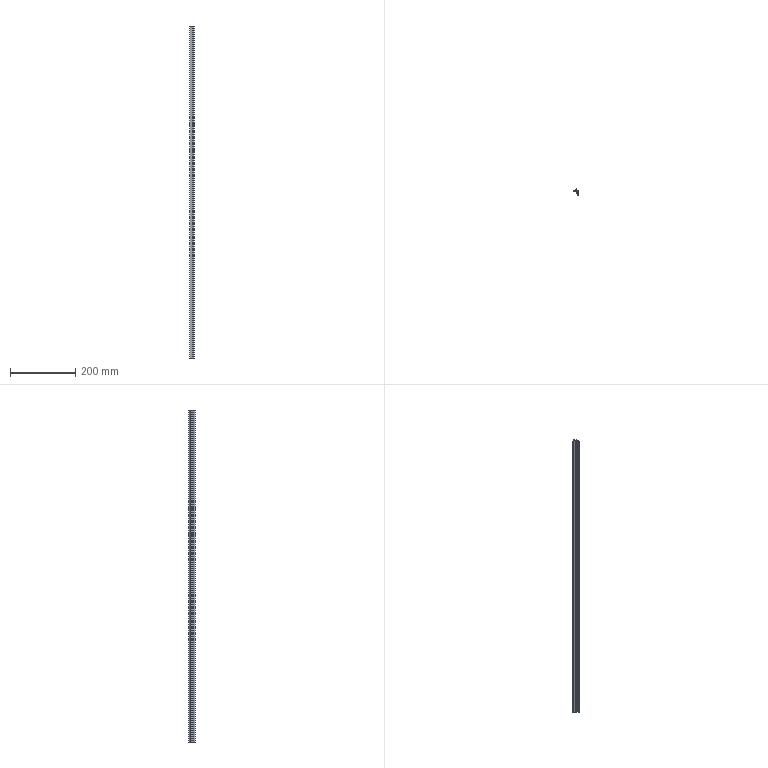Part | SolidWorks | features BaseBody 1, ICE 1, MoveFace 1 | 1 solid | 27 faces | box 14 x 20.3 x 1020 mm | volume 51934 mm3 | plane 20 | cylinder 7 | commonest cylinder face diameters 0.387 x2 0.8 x2 0.4 x1 20 x1 22 x1
STEP:
#1=CARTESIAN_POINT('',(-5.304,-0.625,200.));
#2=VERTEX_POINT('',#1);
#3=CARTESIAN_POINT('',(-5.449,-0.8125,200.));
#4=VERTEX_POINT('',#3);
#5=CARTESIAN_POINT('',(-5.255,-0.8125,200.));
#6=DIRECTION('',(0.,0.,1.));
#7=DIRECTION('',(-1.,0.,0.));
#8=AXIS2_PLACEMENT_3D('',#5,#6,#7);
#9=CIRCLE('',#8,0.1937);
#10=EDGE_CURVE('',#2,#4,#9,.T.);
#11=ORIENTED_EDGE('',*,*,#10,.T.);
#12=CARTESIAN_POINT('',(-5.449,-0.8125,-820.));
#13=VERTEX_POINT('',#12);
#14=CARTESIAN_POINT('',(-5.449,-0.8125,230.));
#15=DIRECTION('',(0.,0.,-1.));
#16=VECTOR('',#15,1000.);
#17=LINE('',#14,#16);
#18=EDGE_CURVE('',#4,#13,#17,.T.);
#19=ORIENTED_EDGE('',*,*,#18,.T.);
#20=CARTESIAN_POINT('',(-5.304,-0.625,-820.));
#21=VERTEX_POINT('',#20);
#22=CARTESIAN_POINT('',(-5.255,-0.8125,-820.));
#23=DIRECTION('',(0.,0.,-1.));
#24=DIRECTION('',(1.,0.,0.));
#25=AXIS2_PLACEMENT_3D('',#22,#23,#24);
#26=CIRCLE('',#25,0.1937);
#27=EDGE_CURVE('',#13,#21,#26,.T.);
#28=ORIENTED_EDGE('',*,*,#27,.T.);
#29=CARTESIAN_POINT('',(-5.304,-0.625,230.));
#30=DIRECTION('',(0.,0.,-1.));
#31=VECTOR('',#30,1000.);
#32=LINE('',#29,#31);
#33=EDGE_CURVE('',#2,#21,#32,.T.);
#34=ORIENTED_EDGE('',*,*,#33,.F.);
#35=EDGE_LOOP('',(#11,#19,#28,#34));
#36=FACE_OUTER_BOUND('',#35,.T.);
#37=CARTESIAN_POINT('',(-5.255,-0.8125,230.));
#38=DIRECTION('',(0.,0.,-1.));
#39=DIRECTION('',(-1.,0.,0.));
#40=AXIS2_PLACEMENT_3D('',#37,#38,#39);
#41=CYLINDRICAL_SURFACE('',#40,0.1937);
#42=ADVANCED_FACE('',(#36),#41,.F.);
#43=CARTESIAN_POINT('',(5.,-1.,-820.));
#44=VERTEX_POINT('',#43);
#45=CARTESIAN_POINT('',(5.,-14.3,-820.));
#46=VERTEX_POINT('',#45);
#47=CARTESIAN_POINT('',(5.,29.623,-820.));
#48=DIRECTION('',(0.,-1.,0.));
#49=VECTOR('',#48,1000.);
#50=LINE('',#47,#49);
#51=EDGE_CURVE('',#44,#46,#50,.T.);
#52=ORIENTED_EDGE('',*,*,#51,.F.);
#53=CARTESIAN_POINT('',(5.,-1.,200.));
#54=VERTEX_POINT('',#53);
#55=CARTESIAN_POINT('',(5.,-1.,230.));
#56=DIRECTION('',(0.,0.,-1.));
#57=VECTOR('',#56,1000.);
#58=LINE('',#55,#57);
#59=EDGE_CURVE('',#54,#44,#58,.T.);
#60=ORIENTED_EDGE('',*,*,#59,.F.);
#61=CARTESIAN_POINT('',(5.,-14.3,200.));
#62=VERTEX_POINT('',#61);
#63=CARTESIAN_POINT('',(5.,-14.3,200.));
#64=DIRECTION('',(0.,1.,0.));
#65=VECTOR('',#64,1000.);
#66=LINE('',#63,#65);
#67=EDGE_CURVE('',#62,#54,#66,.T.);
#68=ORIENTED_EDGE('',*,*,#67,.F.);
#69=CARTESIAN_POINT('',(5.,-14.3,230.));
#70=DIRECTION('',(0.,0.,1.));
#71=VECTOR('',#70,1000.);
#72=LINE('',#69,#71);
#73=EDGE_CURVE('',#46,#62,#72,.T.);
#74=ORIENTED_EDGE('',*,*,#73,.F.);
#75=EDGE_LOOP('',(#52,#60,#68,#74));
#76=FACE_OUTER_BOUND('',#75,.T.);
#77=CARTESIAN_POINT('',(5.,-14.3,230.));
#78=DIRECTION('',(-1.,0.,0.));
#79=DIRECTION('',(0.,0.,1.));
#80=AXIS2_PLACEMENT_3D('',#77,#78,#79);
#81=PLANE('',#80);
#82=ADVANCED_FACE('',(#76),#81,.F.);
#83=CARTESIAN_POINT('',(-9.,-2.,-820.));
#84=VERTEX_POINT('',#83);
#85=CARTESIAN_POINT('',(-9.,-2.,200.));
#86=VERTEX_POINT('',#85);
#87=CARTESIAN_POINT('',(-9.,-2.,230.));
#88=DIRECTION('',(0.,0.,1.));
#89=VECTOR('',#88,1000.);
#90=LINE('',#87,#89);
#91=EDGE_CURVE('',#84,#86,#90,.T.);
#92=ORIENTED_EDGE('',*,*,#91,.F.);
#93=CARTESIAN_POINT('',(0.9,-2.,-820.));
#94=VERTEX_POINT('',#93);
#95=CARTESIAN_POINT('',(5.,-2.,-820.));
#96=DIRECTION('',(-1.,0.,0.));
#97=VECTOR('',#96,1000.);
#98=LINE('',#95,#97);
#99=EDGE_CURVE('',#94,#84,#98,.T.);
#100=ORIENTED_EDGE('',*,*,#99,.F.);
#101=CARTESIAN_POINT('',(0.9,-2.,200.));
#102=VERTEX_POINT('',#101);
#103=CARTESIAN_POINT('',(0.9,-2.,230.));
#104=DIRECTION('',(0.,0.,-1.));
#105=VECTOR('',#104,1000.);
#106=LINE('',#103,#105);
#107=EDGE_CURVE('',#102,#94,#106,.T.);
#108=ORIENTED_EDGE('',*,*,#107,.F.);
#109=CARTESIAN_POINT('',(5.,-2.,200.));
#110=DIRECTION('',(1.,0.,0.));
#111=VECTOR('',#110,1000.);
#112=LINE('',#109,#111);
#113=EDGE_CURVE('',#86,#102,#112,.T.);
#114=ORIENTED_EDGE('',*,*,#113,.F.);
#115=EDGE_LOOP('',(#92,#100,#108,#114));
#116=FACE_OUTER_BOUND('',#115,.T.);
#117=CARTESIAN_POINT('',(-9.,-2.,230.));
#118=DIRECTION('',(0.,1.,0.));
#119=DIRECTION('',(0.,0.,1.));
#120=AXIS2_PLACEMENT_3D('',#117,#118,#119);
#121=PLANE('',#120);
#122=ADVANCED_FACE('',(#116),#121,.F.);
#123=CARTESIAN_POINT('',(4.,-6.,200.));
#124=VERTEX_POINT('',#123);
#125=CARTESIAN_POINT('',(4.,-3.,200.));
#126=VERTEX_POINT('',#125);
#127=CARTESIAN_POINT('',(4.,29.623,200.));
#128=DIRECTION('',(0.,1.,0.));
#129=VECTOR('',#128,1000.);
#130=LINE('',#127,#129);
#131=EDGE_CURVE('',#124,#126,#130,.T.);
#132=ORIENTED_EDGE('',*,*,#131,.F.);
#133=CARTESIAN_POINT('',(1.,-6.,200.));
#134=VERTEX_POINT('',#133);
#135=CARTESIAN_POINT('',(5.,-6.,200.));
#136=DIRECTION('',(1.,0.,0.));
#137=VECTOR('',#136,1000.);
#138=LINE('',#135,#137);
#139=EDGE_CURVE('',#134,#124,#138,.T.);
#140=ORIENTED_EDGE('',*,*,#139,.F.);
#141=CARTESIAN_POINT('',(1.,-6.7,200.));
#142=VERTEX_POINT('',#141);
#143=CARTESIAN_POINT('',(1.,-6.,200.));
#144=DIRECTION('',(0.,-1.,0.));
#145=VECTOR('',#144,1000.);
#146=LINE('',#143,#145);
#147=EDGE_CURVE('',#134,#142,#146,.T.);
#148=ORIENTED_EDGE('',*,*,#147,.T.);
#149=CARTESIAN_POINT('',(-1.7,-6.7,200.));
#150=VERTEX_POINT('',#149);
#151=CARTESIAN_POINT('',(5.,-6.7,200.));
#152=DIRECTION('',(1.,0.,0.));
#153=VECTOR('',#152,1000.);
#154=LINE('',#151,#153);
#155=EDGE_CURVE('',#150,#142,#154,.T.);
#156=ORIENTED_EDGE('',*,*,#155,.F.);
#157=CARTESIAN_POINT('',(-1.7,-7.7,200.));
#158=VERTEX_POINT('',#157);
#159=CARTESIAN_POINT('',(-1.7,-6.7,200.));
#160=DIRECTION('',(0.,-1.,0.));
#161=VECTOR('',#160,1000.);
#162=LINE('',#159,#161);
#163=EDGE_CURVE('',#150,#158,#162,.T.);
#164=ORIENTED_EDGE('',*,*,#163,.T.);
#165=CARTESIAN_POINT('',(4.,-7.7,200.));
#166=VERTEX_POINT('',#165);
#167=CARTESIAN_POINT('',(5.,-7.7,200.));
#168=DIRECTION('',(-1.,0.,0.));
#169=VECTOR('',#168,1000.);
#170=LINE('',#167,#169);
#171=EDGE_CURVE('',#166,#158,#170,.T.);
#172=ORIENTED_EDGE('',*,*,#171,.F.);
#173=CARTESIAN_POINT('',(4.,-14.3,200.));
#174=VERTEX_POINT('',#173);
#175=CARTESIAN_POINT('',(4.,29.623,200.));
#176=DIRECTION('',(0.,1.,0.));
#177=VECTOR('',#176,1000.);
#178=LINE('',#175,#177);
#179=EDGE_CURVE('',#174,#166,#178,.T.);
#180=ORIENTED_EDGE('',*,*,#179,.F.);
#181=CARTESIAN_POINT('',(5.,-14.3,200.));
#182=DIRECTION('',(-1.,0.,0.));
#183=VECTOR('',#182,1000.);
#184=LINE('',#181,#183);
#185=EDGE_CURVE('',#62,#174,#184,.T.);
#186=ORIENTED_EDGE('',*,*,#185,.F.);
#187=ORIENTED_EDGE('',*,*,#67,.T.);
#188=CARTESIAN_POINT('',(-5.207,-1.,200.));
#189=VERTEX_POINT('',#188);
#190=CARTESIAN_POINT('',(5.,-1.,200.));
#191=DIRECTION('',(1.,0.,0.));
#192=VECTOR('',#191,1000.);
#193=LINE('',#190,#192);
#194=EDGE_CURVE('',#189,#54,#193,.T.);
#195=ORIENTED_EDGE('',*,*,#194,.F.);
#196=CARTESIAN_POINT('',(-5.255,-0.8125,200.));
#197=DIRECTION('',(0.,0.,1.));
#198=DIRECTION('',(-1.,0.,0.));
#199=AXIS2_PLACEMENT_3D('',#196,#197,#198);
#200=CIRCLE('',#199,0.1937);
#201=EDGE_CURVE('',#4,#189,#200,.T.);
#202=ORIENTED_EDGE('',*,*,#201,.F.);
#203=ORIENTED_EDGE('',*,*,#10,.F.);
#204=CARTESIAN_POINT('',(-1.368,3.063,200.));
#205=VERTEX_POINT('',#204);
#206=CARTESIAN_POINT('',(-10.628,9.,200.));
#207=DIRECTION('',(0.,0.,1.));
#208=DIRECTION('',(-1.,0.,0.));
#209=AXIS2_PLACEMENT_3D('',#206,#207,#208);
#210=CIRCLE('',#209,11.);
#211=EDGE_CURVE('',#2,#205,#210,.T.);
#212=ORIENTED_EDGE('',*,*,#211,.T.);
#213=CARTESIAN_POINT('',(-1.,2.955,200.));
#214=VERTEX_POINT('',#213);
#215=CARTESIAN_POINT('',(-1.2,2.955,200.));
#216=DIRECTION('',(0.,0.,1.));
#217=DIRECTION('',(-1.,0.,0.));
#218=AXIS2_PLACEMENT_3D('',#215,#216,#217);
#219=CIRCLE('',#218,0.2);
#220=EDGE_CURVE('',#214,#205,#219,.T.);
#221=ORIENTED_EDGE('',*,*,#220,.F.);
#222=CARTESIAN_POINT('',(-1.,1.5,200.));
#223=VERTEX_POINT('',#222);
#224=CARTESIAN_POINT('',(-1.,2.955,200.));
#225=DIRECTION('',(0.,1.,0.));
#226=VECTOR('',#225,1000.);
#227=LINE('',#224,#226);
#228=EDGE_CURVE('',#223,#214,#227,.T.);
#229=ORIENTED_EDGE('',*,*,#228,.F.);
#230=CARTESIAN_POINT('',(0.,1.5,200.));
#231=VERTEX_POINT('',#230);
#232=CARTESIAN_POINT('',(-1.,1.5,200.));
#233=DIRECTION('',(-1.,0.,0.));
#234=VECTOR('',#233,1000.);
#235=LINE('',#232,#234);
#236=EDGE_CURVE('',#231,#223,#235,.T.);
#237=ORIENTED_EDGE('',*,*,#236,.F.);
#238=CARTESIAN_POINT('',(0.,6.,200.));
#239=VERTEX_POINT('',#238);
#240=CARTESIAN_POINT('',(0.,1.5,200.));
#241=DIRECTION('',(0.,-1.,0.));
#242=VECTOR('',#241,1000.);
#243=LINE('',#240,#242);
#244=EDGE_CURVE('',#239,#231,#243,.T.);
#245=ORIENTED_EDGE('',*,*,#244,.F.);
#246=CARTESIAN_POINT('',(-0.8,6.,200.));
#247=VERTEX_POINT('',#246);
#248=CARTESIAN_POINT('',(0.,6.,200.));
#249=DIRECTION('',(1.,0.,0.));
#250=VECTOR('',#249,1000.);
#251=LINE('',#248,#250);
#252=EDGE_CURVE('',#247,#239,#251,.T.);
#253=ORIENTED_EDGE('',*,*,#252,.F.);
#254=CARTESIAN_POINT('',(-1.178,5.731,200.));
#255=VERTEX_POINT('',#254);
#256=CARTESIAN_POINT('',(-0.8,5.6,200.));
#257=DIRECTION('',(0.,0.,1.));
#258=DIRECTION('',(-1.,0.,0.));
#259=AXIS2_PLACEMENT_3D('',#256,#257,#258);
#260=CIRCLE('',#259,0.4);
#261=EDGE_CURVE('',#247,#255,#260,.T.);
#262=ORIENTED_EDGE('',*,*,#261,.T.);
#263=CARTESIAN_POINT('',(-8.678,-0.8077,200.));
#264=VERTEX_POINT('',#263);
#265=CARTESIAN_POINT('',(-10.628,9.,200.));
#266=DIRECTION('',(0.,0.,1.));
#267=DIRECTION('',(-1.,0.,0.));
#268=AXIS2_PLACEMENT_3D('',#265,#266,#267);
#269=CIRCLE('',#268,10.);
#270=EDGE_CURVE('',#264,#255,#269,.T.);
#271=ORIENTED_EDGE('',*,*,#270,.F.);
#272=CARTESIAN_POINT('',(-9.,-1.2,200.));
#273=VERTEX_POINT('',#272);
#274=CARTESIAN_POINT('',(-8.6,-1.2,200.));
#275=DIRECTION('',(0.,0.,1.));
#276=DIRECTION('',(-1.,0.,0.));
#277=AXIS2_PLACEMENT_3D('',#274,#275,#276);
#278=CIRCLE('',#277,0.4);
#279=EDGE_CURVE('',#264,#273,#278,.T.);
#280=ORIENTED_EDGE('',*,*,#279,.T.);
#281=CARTESIAN_POINT('',(-9.,8.,200.));
#282=DIRECTION('',(0.,-1.,0.));
#283=VECTOR('',#282,1000.);
#284=LINE('',#281,#283);
#285=EDGE_CURVE('',#273,#86,#284,.T.);
#286=ORIENTED_EDGE('',*,*,#285,.T.);
#287=ORIENTED_EDGE('',*,*,#113,.T.);
#288=CARTESIAN_POINT('',(0.9,-3.,200.));
#289=VERTEX_POINT('',#288);
#290=CARTESIAN_POINT('',(0.9,29.623,200.));
#291=DIRECTION('',(0.,1.,0.));
#292=VECTOR('',#291,1000.);
#293=LINE('',#290,#292);
#294=EDGE_CURVE('',#289,#102,#293,.T.);
#295=ORIENTED_EDGE('',*,*,#294,.F.);
#296=CARTESIAN_POINT('',(5.,-3.,200.));
#297=DIRECTION('',(-1.,0.,0.));
#298=VECTOR('',#297,1000.);
#299=LINE('',#296,#298);
#300=EDGE_CURVE('',#126,#289,#299,.T.);
#301=ORIENTED_EDGE('',*,*,#300,.F.);
#302=EDGE_LOOP('',(#132,#140,#148,#156,#164,#172,#180,#186,#187,#195,#202,#203,#212,#221,#229,#237,#245,#253,#262,#271,#280,#286,#287,#295,#301));
#303=FACE_OUTER_BOUND('',#302,.T.);
#304=CARTESIAN_POINT('',(5.,29.623,200.));
#305=DIRECTION('',(0.,0.,-1.));
#306=DIRECTION('',(-1.,0.,0.));
#307=AXIS2_PLACEMENT_3D('',#304,#305,#306);
#308=PLANE('',#307);
#309=ADVANCED_FACE('',(#303),#308,.F.);
#310=ORIENTED_EDGE('',*,*,#185,.T.);
#311=CARTESIAN_POINT('',(4.,-14.3,-820.));
#312=VERTEX_POINT('',#311);
#313=CARTESIAN_POINT('',(4.,-14.3,230.));
#314=DIRECTION('',(0.,0.,1.));
#315=VECTOR('',#314,1000.);
#316=LINE('',#313,#315);
#317=EDGE_CURVE('',#312,#174,#316,.T.);
#318=ORIENTED_EDGE('',*,*,#317,.F.);
#319=CARTESIAN_POINT('',(5.,-14.3,-820.));
#320=DIRECTION('',(-1.,0.,0.));
#321=VECTOR('',#320,1000.);
#322=LINE('',#319,#321);
#323=EDGE_CURVE('',#46,#312,#322,.T.);
#324=ORIENTED_EDGE('',*,*,#323,.F.);
#325=ORIENTED_EDGE('',*,*,#73,.T.);
#326=EDGE_LOOP('',(#310,#318,#324,#325));
#327=FACE_OUTER_BOUND('',#326,.T.);
#328=CARTESIAN_POINT('',(4.,-14.3,230.));
#329=DIRECTION('',(0.,1.,0.));
#330=DIRECTION('',(0.,0.,1.));
#331=AXIS2_PLACEMENT_3D('',#328,#329,#330);
#332=PLANE('',#331);
#333=ADVANCED_FACE('',(#327),#332,.F.);
#334=ORIENTED_EDGE('',*,*,#51,.T.);
#335=ORIENTED_EDGE('',*,*,#323,.T.);
#336=CARTESIAN_POINT('',(4.,-7.7,-820.));
#337=VERTEX_POINT('',#336);
#338=CARTESIAN_POINT('',(4.,-7.7,-820.));
#339=DIRECTION('',(0.,-1.,0.));
#340=VECTOR('',#339,1000.);
#341=LINE('',#338,#340);
#342=EDGE_CURVE('',#337,#312,#341,.T.);
#343=ORIENTED_EDGE('',*,*,#342,.F.);
#344=CARTESIAN_POINT('',(-1.7,-7.7,-820.));
#345=VERTEX_POINT('',#344);
#346=CARTESIAN_POINT('',(-1.7,-7.7,-820.));
#347=DIRECTION('',(1.,0.,0.));
#348=VECTOR('',#347,1000.);
#349=LINE('',#346,#348);
#350=EDGE_CURVE('',#345,#337,#349,.T.);
#351=ORIENTED_EDGE('',*,*,#350,.F.);
#352=CARTESIAN_POINT('',(-1.7,-6.7,-820.));
#353=VERTEX_POINT('',#352);
#354=CARTESIAN_POINT('',(-1.7,29.623,-820.));
#355=DIRECTION('',(0.,1.,0.));
#356=VECTOR('',#355,1000.);
#357=LINE('',#354,#356);
#358=EDGE_CURVE('',#345,#353,#357,.T.);
#359=ORIENTED_EDGE('',*,*,#358,.T.);
#360=CARTESIAN_POINT('',(1.,-6.7,-820.));
#361=VERTEX_POINT('',#360);
#362=CARTESIAN_POINT('',(1.,-6.7,-820.));
#363=DIRECTION('',(-1.,0.,0.));
#364=VECTOR('',#363,1000.);
#365=LINE('',#362,#364);
#366=EDGE_CURVE('',#361,#353,#365,.T.);
#367=ORIENTED_EDGE('',*,*,#366,.F.);
#368=CARTESIAN_POINT('',(1.,-6.,-820.));
#369=VERTEX_POINT('',#368);
#370=CARTESIAN_POINT('',(1.,29.623,-820.));
#371=DIRECTION('',(0.,1.,0.));
#372=VECTOR('',#371,1000.);
#373=LINE('',#370,#372);
#374=EDGE_CURVE('',#361,#369,#373,.T.);
#375=ORIENTED_EDGE('',*,*,#374,.T.);
#376=CARTESIAN_POINT('',(4.,-6.,-820.));
#377=VERTEX_POINT('',#376);
#378=CARTESIAN_POINT('',(4.,-6.,-820.));
#379=DIRECTION('',(-1.,0.,0.));
#380=VECTOR('',#379,1000.);
#381=LINE('',#378,#380);
#382=EDGE_CURVE('',#377,#369,#381,.T.);
#383=ORIENTED_EDGE('',*,*,#382,.F.);
#384=CARTESIAN_POINT('',(4.,-3.,-820.));
#385=VERTEX_POINT('',#384);
#386=CARTESIAN_POINT('',(4.,-3.,-820.));
#387=DIRECTION('',(0.,-1.,0.));
#388=VECTOR('',#387,1000.);
#389=LINE('',#386,#388);
#390=EDGE_CURVE('',#385,#377,#389,.T.);
#391=ORIENTED_EDGE('',*,*,#390,.F.);
#392=CARTESIAN_POINT('',(0.9,-3.,-820.));
#393=VERTEX_POINT('',#392);
#394=CARTESIAN_POINT('',(0.9,-3.,-820.));
#395=DIRECTION('',(1.,0.,0.));
#396=VECTOR('',#395,1000.);
#397=LINE('',#394,#396);
#398=EDGE_CURVE('',#393,#385,#397,.T.);
#399=ORIENTED_EDGE('',*,*,#398,.F.);
#400=CARTESIAN_POINT('',(0.9,-2.,-820.));
#401=DIRECTION('',(0.,-1.,0.));
#402=VECTOR('',#401,1000.);
#403=LINE('',#400,#402);
#404=EDGE_CURVE('',#94,#393,#403,.T.);
#405=ORIENTED_EDGE('',*,*,#404,.F.);
#406=ORIENTED_EDGE('',*,*,#99,.T.);
#407=CARTESIAN_POINT('',(-9.,-1.2,-820.));
#408=VERTEX_POINT('',#407);
#409=CARTESIAN_POINT('',(-9.,-1.2,-820.));
#410=DIRECTION('',(0.,-1.,0.));
#411=VECTOR('',#410,1000.);
#412=LINE('',#409,#411);
#413=EDGE_CURVE('',#408,#84,#412,.T.);
#414=ORIENTED_EDGE('',*,*,#413,.F.);
#415=CARTESIAN_POINT('',(-8.678,-0.8077,-820.));
#416=VERTEX_POINT('',#415);
#417=CARTESIAN_POINT('',(-8.6,-1.2,-820.));
#418=DIRECTION('',(0.,0.,-1.));
#419=DIRECTION('',(1.,0.,0.));
#420=AXIS2_PLACEMENT_3D('',#417,#418,#419);
#421=CIRCLE('',#420,0.4);
#422=EDGE_CURVE('',#408,#416,#421,.T.);
#423=ORIENTED_EDGE('',*,*,#422,.T.);
#424=CARTESIAN_POINT('',(-1.178,5.731,-820.));
#425=VERTEX_POINT('',#424);
#426=CARTESIAN_POINT('',(-10.628,9.,-820.));
#427=DIRECTION('',(0.,0.,-1.));
#428=DIRECTION('',(1.,0.,0.));
#429=AXIS2_PLACEMENT_3D('',#426,#427,#428);
#430=CIRCLE('',#429,10.);
#431=EDGE_CURVE('',#425,#416,#430,.T.);
#432=ORIENTED_EDGE('',*,*,#431,.F.);
#433=CARTESIAN_POINT('',(-0.8,6.,-820.));
#434=VERTEX_POINT('',#433);
#435=CARTESIAN_POINT('',(-0.8,5.6,-820.));
#436=DIRECTION('',(0.,0.,-1.));
#437=DIRECTION('',(1.,0.,0.));
#438=AXIS2_PLACEMENT_3D('',#435,#436,#437);
#439=CIRCLE('',#438,0.4);
#440=EDGE_CURVE('',#425,#434,#439,.T.);
#441=ORIENTED_EDGE('',*,*,#440,.T.);
#442=CARTESIAN_POINT('',(0.,6.,-820.));
#443=VERTEX_POINT('',#442);
#444=CARTESIAN_POINT('',(0.,6.,-820.));
#445=DIRECTION('',(-1.,0.,0.));
#446=VECTOR('',#445,1000.);
#447=LINE('',#444,#446);
#448=EDGE_CURVE('',#443,#434,#447,.T.);
#449=ORIENTED_EDGE('',*,*,#448,.F.);
#450=CARTESIAN_POINT('',(0.,1.5,-820.));
#451=VERTEX_POINT('',#450);
#452=CARTESIAN_POINT('',(0.,1.5,-820.));
#453=DIRECTION('',(0.,1.,0.));
#454=VECTOR('',#453,1000.);
#455=LINE('',#452,#454);
#456=EDGE_CURVE('',#451,#443,#455,.T.);
#457=ORIENTED_EDGE('',*,*,#456,.F.);
#458=CARTESIAN_POINT('',(-1.,1.5,-820.));
#459=VERTEX_POINT('',#458);
#460=CARTESIAN_POINT('',(-1.,1.5,-820.));
#461=DIRECTION('',(1.,0.,0.));
#462=VECTOR('',#461,1000.);
#463=LINE('',#460,#462);
#464=EDGE_CURVE('',#459,#451,#463,.T.);
#465=ORIENTED_EDGE('',*,*,#464,.F.);
#466=CARTESIAN_POINT('',(-1.,2.955,-820.));
#467=VERTEX_POINT('',#466);
#468=CARTESIAN_POINT('',(-1.,2.955,-820.));
#469=DIRECTION('',(0.,-1.,0.));
#470=VECTOR('',#469,1000.);
#471=LINE('',#468,#470);
#472=EDGE_CURVE('',#467,#459,#471,.T.);
#473=ORIENTED_EDGE('',*,*,#472,.F.);
#474=CARTESIAN_POINT('',(-1.368,3.063,-820.));
#475=VERTEX_POINT('',#474);
#476=CARTESIAN_POINT('',(-1.2,2.955,-820.));
#477=DIRECTION('',(0.,0.,-1.));
#478=DIRECTION('',(1.,0.,0.));
#479=AXIS2_PLACEMENT_3D('',#476,#477,#478);
#480=CIRCLE('',#479,0.2);
#481=EDGE_CURVE('',#475,#467,#480,.T.);
#482=ORIENTED_EDGE('',*,*,#481,.F.);
#483=CARTESIAN_POINT('',(-10.628,9.,-820.));
#484=DIRECTION('',(0.,0.,-1.));
#485=DIRECTION('',(1.,0.,0.));
#486=AXIS2_PLACEMENT_3D('',#483,#484,#485);
#487=CIRCLE('',#486,11.);
#488=EDGE_CURVE('',#475,#21,#487,.T.);
#489=ORIENTED_EDGE('',*,*,#488,.T.);
#490=ORIENTED_EDGE('',*,*,#27,.F.);
#491=CARTESIAN_POINT('',(-5.207,-1.,-820.));
#492=VERTEX_POINT('',#491);
#493=CARTESIAN_POINT('',(-5.255,-0.8125,-820.));
#494=DIRECTION('',(0.,0.,-1.));
#495=DIRECTION('',(1.,0.,0.));
#496=AXIS2_PLACEMENT_3D('',#493,#494,#495);
#497=CIRCLE('',#496,0.1937);
#498=EDGE_CURVE('',#492,#13,#497,.T.);
#499=ORIENTED_EDGE('',*,*,#498,.F.);
#500=CARTESIAN_POINT('',(5.,-1.,-820.));
#501=DIRECTION('',(-1.,0.,0.));
#502=VECTOR('',#501,1000.);
#503=LINE('',#500,#502);
#504=EDGE_CURVE('',#44,#492,#503,.T.);
#505=ORIENTED_EDGE('',*,*,#504,.F.);
#506=EDGE_LOOP('',(#334,#335,#343,#351,#359,#367,#375,#383,#391,#399,#405,#406,#414,#423,#432,#441,#449,#457,#465,#473,#482,#489,#490,#499,#505));
#507=FACE_OUTER_BOUND('',#506,.T.);
#508=CARTESIAN_POINT('',(5.,29.623,-820.));
#509=DIRECTION('',(0.,0.,1.));
#510=DIRECTION('',(1.,0.,0.));
#511=AXIS2_PLACEMENT_3D('',#508,#509,#510);
#512=PLANE('',#511);
#513=ADVANCED_FACE('',(#507),#512,.F.);
#514=ORIENTED_EDGE('',*,*,#59,.T.);
#515=ORIENTED_EDGE('',*,*,#504,.T.);
#516=CARTESIAN_POINT('',(-5.207,-1.,230.));
#517=DIRECTION('',(0.,0.,-1.));
#518=VECTOR('',#517,1000.);
#519=LINE('',#516,#518);
#520=EDGE_CURVE('',#189,#492,#519,.T.);
#521=ORIENTED_EDGE('',*,*,#520,.F.);
#522=ORIENTED_EDGE('',*,*,#194,.T.);
#523=EDGE_LOOP('',(#514,#515,#521,#522));
#524=FACE_OUTER_BOUND('',#523,.T.);
#525=CARTESIAN_POINT('',(5.,-1.,230.));
#526=DIRECTION('',(0.,-1.,0.));
#527=DIRECTION('',(0.,0.,-1.));
#528=AXIS2_PLACEMENT_3D('',#525,#526,#527);
#529=PLANE('',#528);
#530=ADVANCED_FACE('',(#524),#529,.F.);
#531=CARTESIAN_POINT('',(-9.,-1.2,230.));
#532=DIRECTION('',(0.,0.,1.));
#533=VECTOR('',#532,1000.);
#534=LINE('',#531,#533);
#535=EDGE_CURVE('',#408,#273,#534,.T.);
#536=ORIENTED_EDGE('',*,*,#535,.F.);
#537=ORIENTED_EDGE('',*,*,#413,.T.);
#538=ORIENTED_EDGE('',*,*,#91,.T.);
#539=ORIENTED_EDGE('',*,*,#285,.F.);
#540=EDGE_LOOP('',(#536,#537,#538,#539));
#541=FACE_OUTER_BOUND('',#540,.T.);
#542=CARTESIAN_POINT('',(-9.,-1.2,230.));
#543=DIRECTION('',(1.,0.,0.));
#544=DIRECTION('',(0.,0.,-1.));
#545=AXIS2_PLACEMENT_3D('',#542,#543,#544);
#546=PLANE('',#545);
#547=ADVANCED_FACE('',(#541),#546,.F.);
#548=ORIENTED_EDGE('',*,*,#294,.T.);
#549=ORIENTED_EDGE('',*,*,#107,.T.);
#550=ORIENTED_EDGE('',*,*,#404,.T.);
#551=CARTESIAN_POINT('',(0.9,-3.,230.));
#552=DIRECTION('',(0.,0.,-1.));
#553=VECTOR('',#552,1000.);
#554=LINE('',#551,#553);
#555=EDGE_CURVE('',#289,#393,#554,.T.);
#556=ORIENTED_EDGE('',*,*,#555,.F.);
#557=EDGE_LOOP('',(#548,#549,#550,#556));
#558=FACE_OUTER_BOUND('',#557,.T.);
#559=CARTESIAN_POINT('',(0.9,-2.,230.));
#560=DIRECTION('',(1.,0.,0.));
#561=DIRECTION('',(0.,0.,-1.));
#562=AXIS2_PLACEMENT_3D('',#559,#560,#561);
#563=PLANE('',#562);
#564=ADVANCED_FACE('',(#558),#563,.F.);
#565=ORIENTED_EDGE('',*,*,#300,.T.);
#566=ORIENTED_EDGE('',*,*,#555,.T.);
#567=ORIENTED_EDGE('',*,*,#398,.T.);
#568=CARTESIAN_POINT('',(4.,-3.,230.));
#569=DIRECTION('',(0.,0.,-1.));
#570=VECTOR('',#569,1000.);
#571=LINE('',#568,#570);
#572=EDGE_CURVE('',#126,#385,#571,.T.);
#573=ORIENTED_EDGE('',*,*,#572,.F.);
#574=EDGE_LOOP('',(#565,#566,#567,#573));
#575=FACE_OUTER_BOUND('',#574,.T.);
#576=CARTESIAN_POINT('',(0.9,-3.,230.));
#577=DIRECTION('',(0.,1.,0.));
#578=DIRECTION('',(0.,0.,1.));
#579=AXIS2_PLACEMENT_3D('',#576,#577,#578);
#580=PLANE('',#579);
#581=ADVANCED_FACE('',(#575),#580,.F.);
#582=ORIENTED_EDGE('',*,*,#131,.T.);
#583=ORIENTED_EDGE('',*,*,#572,.T.);
#584=ORIENTED_EDGE('',*,*,#390,.T.);
#585=CARTESIAN_POINT('',(4.,-6.,230.));
#586=DIRECTION('',(0.,0.,-1.));
#587=VECTOR('',#586,1000.);
#588=LINE('',#585,#587);
#589=EDGE_CURVE('',#124,#377,#588,.T.);
#590=ORIENTED_EDGE('',*,*,#589,.F.);
#591=EDGE_LOOP('',(#582,#583,#584,#590));
#592=FACE_OUTER_BOUND('',#591,.T.);
#593=CARTESIAN_POINT('',(4.,-3.,230.));
#594=DIRECTION('',(1.,0.,0.));
#595=DIRECTION('',(0.,0.,-1.));
#596=AXIS2_PLACEMENT_3D('',#593,#594,#595);
#597=PLANE('',#596);
#598=ADVANCED_FACE('',(#592),#597,.F.);
#599=ORIENTED_EDGE('',*,*,#139,.T.);
#600=ORIENTED_EDGE('',*,*,#589,.T.);
#601=ORIENTED_EDGE('',*,*,#382,.T.);
#602=CARTESIAN_POINT('',(1.,-6.,230.));
#603=DIRECTION('',(0.,0.,-1.));
#604=VECTOR('',#603,1000.);
#605=LINE('',#602,#604);
#606=EDGE_CURVE('',#134,#369,#605,.T.);
#607=ORIENTED_EDGE('',*,*,#606,.F.);
#608=EDGE_LOOP('',(#599,#600,#601,#607));
#609=FACE_OUTER_BOUND('',#608,.T.);
#610=CARTESIAN_POINT('',(4.,-6.,230.));
#611=DIRECTION('',(0.,-1.,0.));
#612=DIRECTION('',(0.,0.,-1.));
#613=AXIS2_PLACEMENT_3D('',#610,#611,#612);
#614=PLANE('',#613);
#615=ADVANCED_FACE('',(#609),#614,.F.);
#616=ORIENTED_EDGE('',*,*,#155,.T.);
#617=CARTESIAN_POINT('',(1.,-6.7,230.));
#618=DIRECTION('',(0.,0.,1.));
#619=VECTOR('',#618,1000.);
#620=LINE('',#617,#619);
#621=EDGE_CURVE('',#361,#142,#620,.T.);
#622=ORIENTED_EDGE('',*,*,#621,.F.);
#623=ORIENTED_EDGE('',*,*,#366,.T.);
#624=CARTESIAN_POINT('',(-1.7,-6.7,230.));
#625=DIRECTION('',(0.,0.,-1.));
#626=VECTOR('',#625,1000.);
#627=LINE('',#624,#626);
#628=EDGE_CURVE('',#150,#353,#627,.T.);
#629=ORIENTED_EDGE('',*,*,#628,.F.);
#630=EDGE_LOOP('',(#616,#622,#623,#629));
#631=FACE_OUTER_BOUND('',#630,.T.);
#632=CARTESIAN_POINT('',(1.,-6.7,230.));
#633=DIRECTION('',(0.,-1.,0.));
#634=DIRECTION('',(0.,0.,-1.));
#635=AXIS2_PLACEMENT_3D('',#632,#633,#634);
#636=PLANE('',#635);
#637=ADVANCED_FACE('',(#631),#636,.F.);
#638=ORIENTED_EDGE('',*,*,#171,.T.);
#639=CARTESIAN_POINT('',(-1.7,-7.7,230.));
#640=DIRECTION('',(0.,0.,1.));
#641=VECTOR('',#640,1000.);
#642=LINE('',#639,#641);
#643=EDGE_CURVE('',#345,#158,#642,.T.);
#644=ORIENTED_EDGE('',*,*,#643,.F.);
#645=ORIENTED_EDGE('',*,*,#350,.T.);
#646=CARTESIAN_POINT('',(4.,-7.7,230.));
#647=DIRECTION('',(0.,0.,-1.));
#648=VECTOR('',#647,1000.);
#649=LINE('',#646,#648);
#650=EDGE_CURVE('',#166,#337,#649,.T.);
#651=ORIENTED_EDGE('',*,*,#650,.F.);
#652=EDGE_LOOP('',(#638,#644,#645,#651));
#653=FACE_OUTER_BOUND('',#652,.T.);
#654=CARTESIAN_POINT('',(-1.7,-7.7,230.));
#655=DIRECTION('',(0.,1.,0.));
#656=DIRECTION('',(0.,0.,1.));
#657=AXIS2_PLACEMENT_3D('',#654,#655,#656);
#658=PLANE('',#657);
#659=ADVANCED_FACE('',(#653),#658,.F.);
#660=ORIENTED_EDGE('',*,*,#179,.T.);
#661=ORIENTED_EDGE('',*,*,#650,.T.);
#662=ORIENTED_EDGE('',*,*,#342,.T.);
#663=ORIENTED_EDGE('',*,*,#317,.T.);
#664=EDGE_LOOP('',(#660,#661,#662,#663));
#665=FACE_OUTER_BOUND('',#664,.T.);
#666=CARTESIAN_POINT('',(4.,-7.7,230.));
#667=DIRECTION('',(1.,0.,0.));
#668=DIRECTION('',(0.,0.,-1.));
#669=AXIS2_PLACEMENT_3D('',#666,#667,#668);
#670=PLANE('',#669);
#671=ADVANCED_FACE('',(#665),#670,.F.);
#672=ORIENTED_EDGE('',*,*,#18,.F.);
#673=ORIENTED_EDGE('',*,*,#201,.T.);
#674=ORIENTED_EDGE('',*,*,#520,.T.);
#675=ORIENTED_EDGE('',*,*,#498,.T.);
#676=EDGE_LOOP('',(#672,#673,#674,#675));
#677=FACE_OUTER_BOUND('',#676,.T.);
#678=CARTESIAN_POINT('',(-5.255,-0.8125,230.));
#679=DIRECTION('',(0.,0.,-1.));
#680=DIRECTION('',(-1.,0.,0.));
#681=AXIS2_PLACEMENT_3D('',#678,#679,#680);
#682=CYLINDRICAL_SURFACE('',#681,0.1937);
#683=ADVANCED_FACE('',(#677),#682,.F.);
#684=CARTESIAN_POINT('',(-1.,2.955,230.));
#685=DIRECTION('',(0.,0.,1.));
#686=VECTOR('',#685,1000.);
#687=LINE('',#684,#686);
#688=EDGE_CURVE('',#467,#214,#687,.T.);
#689=ORIENTED_EDGE('',*,*,#688,.F.);
#690=ORIENTED_EDGE('',*,*,#472,.T.);
#691=CARTESIAN_POINT('',(-1.,1.5,230.));
#692=DIRECTION('',(0.,0.,-1.));
#693=VECTOR('',#692,1000.);
#694=LINE('',#691,#693);
#695=EDGE_CURVE('',#223,#459,#694,.T.);
#696=ORIENTED_EDGE('',*,*,#695,.F.);
#697=ORIENTED_EDGE('',*,*,#228,.T.);
#698=EDGE_LOOP('',(#689,#690,#696,#697));
#699=FACE_OUTER_BOUND('',#698,.T.);
#700=CARTESIAN_POINT('',(-1.,2.955,230.));
#701=DIRECTION('',(1.,0.,0.));
#702=DIRECTION('',(0.,0.,-1.));
#703=AXIS2_PLACEMENT_3D('',#700,#701,#702);
#704=PLANE('',#703);
#705=ADVANCED_FACE('',(#699),#704,.F.);
#706=ORIENTED_EDGE('',*,*,#488,.F.);
#707=CARTESIAN_POINT('',(-1.368,3.063,230.));
#708=DIRECTION('',(0.,0.,1.));
#709=VECTOR('',#708,1000.);
#710=LINE('',#707,#709);
#711=EDGE_CURVE('',#475,#205,#710,.T.);
#712=ORIENTED_EDGE('',*,*,#711,.T.);
#713=ORIENTED_EDGE('',*,*,#211,.F.);
#714=ORIENTED_EDGE('',*,*,#33,.T.);
#715=EDGE_LOOP('',(#706,#712,#713,#714));
#716=FACE_OUTER_BOUND('',#715,.T.);
#717=CARTESIAN_POINT('',(-10.628,9.,230.));
#718=DIRECTION('',(0.,0.,-1.));
#719=DIRECTION('',(-1.,0.,0.));
#720=AXIS2_PLACEMENT_3D('',#717,#718,#719);
#721=CYLINDRICAL_SURFACE('',#720,11.);
#722=ADVANCED_FACE('',(#716),#721,.T.);
#723=CARTESIAN_POINT('',(-1.178,5.731,230.));
#724=DIRECTION('',(0.,0.,1.));
#725=VECTOR('',#724,1000.);
#726=LINE('',#723,#725);
#727=EDGE_CURVE('',#425,#255,#726,.T.);
#728=ORIENTED_EDGE('',*,*,#727,.F.);
#729=ORIENTED_EDGE('',*,*,#431,.T.);
#730=CARTESIAN_POINT('',(-8.678,-0.8077,230.));
#731=DIRECTION('',(0.,0.,-1.));
#732=VECTOR('',#731,1000.);
#733=LINE('',#730,#732);
#734=EDGE_CURVE('',#264,#416,#733,.T.);
#735=ORIENTED_EDGE('',*,*,#734,.F.);
#736=ORIENTED_EDGE('',*,*,#270,.T.);
#737=EDGE_LOOP('',(#728,#729,#735,#736));
#738=FACE_OUTER_BOUND('',#737,.T.);
#739=CARTESIAN_POINT('',(-10.628,9.,230.));
#740=DIRECTION('',(0.,0.,-1.));
#741=DIRECTION('',(-1.,0.,0.));
#742=AXIS2_PLACEMENT_3D('',#739,#740,#741);
#743=CYLINDRICAL_SURFACE('',#742,10.);
#744=ADVANCED_FACE('',(#738),#743,.F.);
#745=CARTESIAN_POINT('',(0.,1.5,230.));
#746=DIRECTION('',(0.,0.,1.));
#747=VECTOR('',#746,1000.);
#748=LINE('',#745,#747);
#749=EDGE_CURVE('',#451,#231,#748,.T.);
#750=ORIENTED_EDGE('',*,*,#749,.F.);
#751=ORIENTED_EDGE('',*,*,#456,.T.);
#752=CARTESIAN_POINT('',(0.,6.,230.));
#753=DIRECTION('',(0.,0.,-1.));
#754=VECTOR('',#753,1000.);
#755=LINE('',#752,#754);
#756=EDGE_CURVE('',#239,#443,#755,.T.);
#757=ORIENTED_EDGE('',*,*,#756,.F.);
#758=ORIENTED_EDGE('',*,*,#244,.T.);
#759=EDGE_LOOP('',(#750,#751,#757,#758));
#760=FACE_OUTER_BOUND('',#759,.T.);
#761=CARTESIAN_POINT('',(0.,1.5,230.));
#762=DIRECTION('',(-1.,0.,0.));
#763=DIRECTION('',(0.,0.,1.));
#764=AXIS2_PLACEMENT_3D('',#761,#762,#763);
#765=PLANE('',#764);
#766=ADVANCED_FACE('',(#760),#765,.F.);
#767=ORIENTED_EDGE('',*,*,#422,.F.);
#768=ORIENTED_EDGE('',*,*,#535,.T.);
#769=ORIENTED_EDGE('',*,*,#279,.F.);
#770=ORIENTED_EDGE('',*,*,#734,.T.);
#771=EDGE_LOOP('',(#767,#768,#769,#770));
#772=FACE_OUTER_BOUND('',#771,.T.);
#773=CARTESIAN_POINT('',(-8.6,-1.2,230.));
#774=DIRECTION('',(0.,0.,-1.));
#775=DIRECTION('',(-1.,0.,0.));
#776=AXIS2_PLACEMENT_3D('',#773,#774,#775);
#777=CYLINDRICAL_SURFACE('',#776,0.4);
#778=ADVANCED_FACE('',(#772),#777,.T.);
#779=ORIENTED_EDGE('',*,*,#147,.F.);
#780=ORIENTED_EDGE('',*,*,#606,.T.);
#781=ORIENTED_EDGE('',*,*,#374,.F.);
#782=ORIENTED_EDGE('',*,*,#621,.T.);
#783=EDGE_LOOP('',(#779,#780,#781,#782));
#784=FACE_OUTER_BOUND('',#783,.T.);
#785=CARTESIAN_POINT('',(1.,-6.,230.));
#786=DIRECTION('',(1.,0.,0.));
#787=DIRECTION('',(0.,0.,-1.));
#788=AXIS2_PLACEMENT_3D('',#785,#786,#787);
#789=PLANE('',#788);
#790=ADVANCED_FACE('',(#784),#789,.F.);
#791=ORIENTED_EDGE('',*,*,#163,.F.);
#792=ORIENTED_EDGE('',*,*,#628,.T.);
#793=ORIENTED_EDGE('',*,*,#358,.F.);
#794=ORIENTED_EDGE('',*,*,#643,.T.);
#795=EDGE_LOOP('',(#791,#792,#793,#794));
#796=FACE_OUTER_BOUND('',#795,.T.);
#797=CARTESIAN_POINT('',(-1.7,-6.7,230.));
#798=DIRECTION('',(1.,0.,0.));
#799=DIRECTION('',(0.,0.,-1.));
#800=AXIS2_PLACEMENT_3D('',#797,#798,#799);
#801=PLANE('',#800);
#802=ADVANCED_FACE('',(#796),#801,.F.);
#803=ORIENTED_EDGE('',*,*,#711,.F.);
#804=ORIENTED_EDGE('',*,*,#481,.T.);
#805=ORIENTED_EDGE('',*,*,#688,.T.);
#806=ORIENTED_EDGE('',*,*,#220,.T.);
#807=EDGE_LOOP('',(#803,#804,#805,#806));
#808=FACE_OUTER_BOUND('',#807,.T.);
#809=CARTESIAN_POINT('',(-1.2,2.955,230.));
#810=DIRECTION('',(0.,0.,-1.));
#811=DIRECTION('',(-1.,0.,0.));
#812=AXIS2_PLACEMENT_3D('',#809,#810,#811);
#813=CYLINDRICAL_SURFACE('',#812,0.2);
#814=ADVANCED_FACE('',(#808),#813,.F.);
#815=ORIENTED_EDGE('',*,*,#695,.T.);
#816=ORIENTED_EDGE('',*,*,#464,.T.);
#817=ORIENTED_EDGE('',*,*,#749,.T.);
#818=ORIENTED_EDGE('',*,*,#236,.T.);
#819=EDGE_LOOP('',(#815,#816,#817,#818));
#820=FACE_OUTER_BOUND('',#819,.T.);
#821=CARTESIAN_POINT('',(-1.,1.5,230.));
#822=DIRECTION('',(0.,1.,0.));
#823=DIRECTION('',(0.,0.,1.));
#824=AXIS2_PLACEMENT_3D('',#821,#822,#823);
#825=PLANE('',#824);
#826=ADVANCED_FACE('',(#820),#825,.F.);
#827=ORIENTED_EDGE('',*,*,#440,.F.);
#828=ORIENTED_EDGE('',*,*,#727,.T.);
#829=ORIENTED_EDGE('',*,*,#261,.F.);
#830=CARTESIAN_POINT('',(-0.8,6.,230.));
#831=DIRECTION('',(0.,0.,-1.));
#832=VECTOR('',#831,1000.);
#833=LINE('',#830,#832);
#834=EDGE_CURVE('',#247,#434,#833,.T.);
#835=ORIENTED_EDGE('',*,*,#834,.T.);
#836=EDGE_LOOP('',(#827,#828,#829,#835));
#837=FACE_OUTER_BOUND('',#836,.T.);
#838=CARTESIAN_POINT('',(-0.8,5.6,230.));
#839=DIRECTION('',(0.,0.,-1.));
#840=DIRECTION('',(-1.,0.,0.));
#841=AXIS2_PLACEMENT_3D('',#838,#839,#840);
#842=CYLINDRICAL_SURFACE('',#841,0.4);
#843=ADVANCED_FACE('',(#837),#842,.T.);
#844=ORIENTED_EDGE('',*,*,#756,.T.);
#845=ORIENTED_EDGE('',*,*,#448,.T.);
#846=ORIENTED_EDGE('',*,*,#834,.F.);
#847=ORIENTED_EDGE('',*,*,#252,.T.);
#848=EDGE_LOOP('',(#844,#845,#846,#847));
#849=FACE_OUTER_BOUND('',#848,.T.);
#850=CARTESIAN_POINT('',(0.,6.,230.));
#851=DIRECTION('',(0.,-1.,0.));
#852=DIRECTION('',(0.,0.,-1.));
#853=AXIS2_PLACEMENT_3D('',#850,#851,#852);
#854=PLANE('',#853);
#855=ADVANCED_FACE('',(#849),#854,.F.);
#856=CLOSED_SHELL('',(#42,#82,#122,#309,#333,#513,#530,#547,#564,#581,#598,#615,#637,#659,#671,#683,#705,#722,#744,#766,#778,#790,#802,#814,#826,#843,#855));
#857=MANIFOLD_SOLID_BREP('',#856);
#858=CARTESIAN_POINT('',(0.,0.,0.));
#859=DIRECTION('',(0.,0.,1.));
#860=DIRECTION('',(1.,0.,0.));
#861=AXIS2_PLACEMENT_3D('',#858,#859,#860);
#862=(LENGTH_UNIT()NAMED_UNIT(*)SI_UNIT(.MILLI.,.METRE.));
#863=UNCERTAINTY_MEASURE_WITH_UNIT(LENGTH_MEASURE(0.00001),#862,'','');
#864=(NAMED_UNIT(*)PLANE_ANGLE_UNIT()SI_UNIT($,.RADIAN.));
#865=(NAMED_UNIT(*)SI_UNIT($,.STERADIAN.)SOLID_ANGLE_UNIT());
#866=(GEOMETRIC_REPRESENTATION_CONTEXT(3)GLOBAL_UNCERTAINTY_ASSIGNED_CONTEXT((#863))GLOBAL_UNIT_ASSIGNED_CONTEXT((#862,#864,#865))REPRESENTATION_CONTEXT('',''));
#867=ADVANCED_BREP_SHAPE_REPRESENTATION('',(#857,#861),#866);